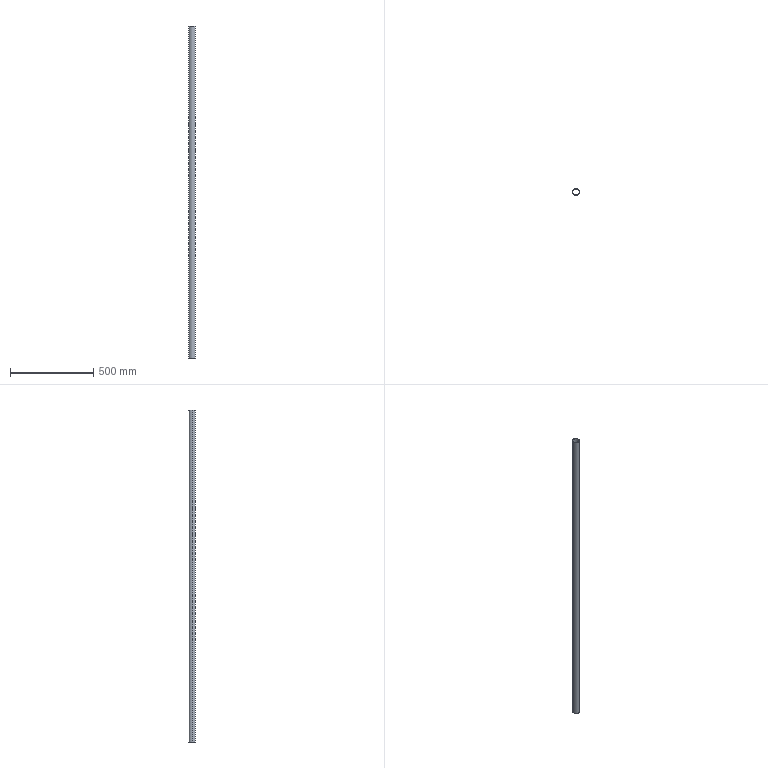Part | SolidWorks | features Extrusion 1 | 1 solid | 6 faces | box 42 x 42 x 2000 mm | volume 502655 mm3 | cylinder 4 | plane 2 | commonest cylinder face diameters 38 x2 42 x2
STEP:
#1=CARTESIAN_POINT('',(-19.,0.,2000.));
#2=VERTEX_POINT('',#1);
#3=CARTESIAN_POINT('',(19.,0.,2000.));
#4=VERTEX_POINT('',#3);
#5=CARTESIAN_POINT('',(0.,0.,2000.));
#6=DIRECTION('',(0.,0.,1.));
#7=DIRECTION('',(1.,0.,0.));
#8=AXIS2_PLACEMENT_3D('',#5,#6,#7);
#9=CIRCLE('',#8,19.);
#10=EDGE_CURVE('',#2,#4,#9,.T.);
#11=ORIENTED_EDGE('',*,*,#10,.T.);
#12=CARTESIAN_POINT('',(19.,0.,0.));
#13=VERTEX_POINT('',#12);
#14=CARTESIAN_POINT('',(19.,0.,2000.));
#15=DIRECTION('',(0.,0.,-1.));
#16=VECTOR('',#15,1000.);
#17=LINE('',#14,#16);
#18=EDGE_CURVE('',#4,#13,#17,.T.);
#19=ORIENTED_EDGE('',*,*,#18,.T.);
#20=CARTESIAN_POINT('',(-19.,0.,0.));
#21=VERTEX_POINT('',#20);
#22=CARTESIAN_POINT('',(0.,0.,0.));
#23=DIRECTION('',(0.,0.,1.));
#24=DIRECTION('',(1.,0.,0.));
#25=AXIS2_PLACEMENT_3D('',#22,#23,#24);
#26=CIRCLE('',#25,19.);
#27=EDGE_CURVE('',#21,#13,#26,.T.);
#28=ORIENTED_EDGE('',*,*,#27,.F.);
#29=CARTESIAN_POINT('',(-19.,0.,2000.));
#30=DIRECTION('',(0.,0.,-1.));
#31=VECTOR('',#30,1000.);
#32=LINE('',#29,#31);
#33=EDGE_CURVE('',#2,#21,#32,.T.);
#34=ORIENTED_EDGE('',*,*,#33,.F.);
#35=EDGE_LOOP('',(#11,#19,#28,#34));
#36=FACE_OUTER_BOUND('',#35,.T.);
#37=CARTESIAN_POINT('',(0.,0.,2000.));
#38=DIRECTION('',(0.,0.,-1.));
#39=DIRECTION('',(-1.,0.,0.));
#40=AXIS2_PLACEMENT_3D('',#37,#38,#39);
#41=CYLINDRICAL_SURFACE('',#40,19.);
#42=ADVANCED_FACE('',(#36),#41,.F.);
#43=CARTESIAN_POINT('',(21.,0.,2000.));
#44=VERTEX_POINT('',#43);
#45=CARTESIAN_POINT('',(-21.,0.,2000.));
#46=VERTEX_POINT('',#45);
#47=CARTESIAN_POINT('',(0.,0.,2000.));
#48=DIRECTION('',(0.,0.,1.));
#49=DIRECTION('',(1.,0.,0.));
#50=AXIS2_PLACEMENT_3D('',#47,#48,#49);
#51=CIRCLE('',#50,21.);
#52=EDGE_CURVE('',#44,#46,#51,.T.);
#53=ORIENTED_EDGE('',*,*,#52,.F.);
#54=CARTESIAN_POINT('',(21.,0.,0.));
#55=VERTEX_POINT('',#54);
#56=CARTESIAN_POINT('',(21.,0.,2000.));
#57=DIRECTION('',(0.,0.,-1.));
#58=VECTOR('',#57,1000.);
#59=LINE('',#56,#58);
#60=EDGE_CURVE('',#44,#55,#59,.T.);
#61=ORIENTED_EDGE('',*,*,#60,.T.);
#62=CARTESIAN_POINT('',(-21.,0.,0.));
#63=VERTEX_POINT('',#62);
#64=CARTESIAN_POINT('',(0.,0.,0.));
#65=DIRECTION('',(0.,0.,1.));
#66=DIRECTION('',(1.,0.,0.));
#67=AXIS2_PLACEMENT_3D('',#64,#65,#66);
#68=CIRCLE('',#67,21.);
#69=EDGE_CURVE('',#55,#63,#68,.T.);
#70=ORIENTED_EDGE('',*,*,#69,.T.);
#71=CARTESIAN_POINT('',(-21.,0.,2000.));
#72=DIRECTION('',(0.,0.,-1.));
#73=VECTOR('',#72,1000.);
#74=LINE('',#71,#73);
#75=EDGE_CURVE('',#46,#63,#74,.T.);
#76=ORIENTED_EDGE('',*,*,#75,.F.);
#77=EDGE_LOOP('',(#53,#61,#70,#76));
#78=FACE_OUTER_BOUND('',#77,.T.);
#79=CARTESIAN_POINT('',(0.,0.,2000.));
#80=DIRECTION('',(0.,0.,-1.));
#81=DIRECTION('',(-1.,0.,0.));
#82=AXIS2_PLACEMENT_3D('',#79,#80,#81);
#83=CYLINDRICAL_SURFACE('',#82,21.);
#84=ADVANCED_FACE('',(#78),#83,.T.);
#85=CARTESIAN_POINT('',(0.,0.,2000.));
#86=DIRECTION('',(0.,0.,1.));
#87=DIRECTION('',(1.,0.,0.));
#88=AXIS2_PLACEMENT_3D('',#85,#86,#87);
#89=CIRCLE('',#88,21.);
#90=EDGE_CURVE('',#46,#44,#89,.T.);
#91=ORIENTED_EDGE('',*,*,#90,.T.);
#92=ORIENTED_EDGE('',*,*,#52,.T.);
#93=EDGE_LOOP('',(#91,#92));
#94=FACE_OUTER_BOUND('',#93,.T.);
#95=ORIENTED_EDGE('',*,*,#10,.F.);
#96=CARTESIAN_POINT('',(0.,0.,2000.));
#97=DIRECTION('',(0.,0.,1.));
#98=DIRECTION('',(1.,0.,0.));
#99=AXIS2_PLACEMENT_3D('',#96,#97,#98);
#100=CIRCLE('',#99,19.);
#101=EDGE_CURVE('',#4,#2,#100,.T.);
#102=ORIENTED_EDGE('',*,*,#101,.F.);
#103=EDGE_LOOP('',(#95,#102));
#104=FACE_BOUND('',#103,.T.);
#105=CARTESIAN_POINT('',(0.,0.,2000.));
#106=DIRECTION('',(0.,0.,1.));
#107=DIRECTION('',(1.,0.,0.));
#108=AXIS2_PLACEMENT_3D('',#105,#106,#107);
#109=PLANE('',#108);
#110=ADVANCED_FACE('',(#94,#104),#109,.T.);
#111=CARTESIAN_POINT('',(0.,0.,0.));
#112=DIRECTION('',(0.,0.,1.));
#113=DIRECTION('',(1.,0.,0.));
#114=AXIS2_PLACEMENT_3D('',#111,#112,#113);
#115=CIRCLE('',#114,21.);
#116=EDGE_CURVE('',#63,#55,#115,.T.);
#117=ORIENTED_EDGE('',*,*,#116,.F.);
#118=ORIENTED_EDGE('',*,*,#69,.F.);
#119=EDGE_LOOP('',(#117,#118));
#120=FACE_OUTER_BOUND('',#119,.T.);
#121=ORIENTED_EDGE('',*,*,#27,.T.);
#122=CARTESIAN_POINT('',(0.,0.,0.));
#123=DIRECTION('',(0.,0.,1.));
#124=DIRECTION('',(1.,0.,0.));
#125=AXIS2_PLACEMENT_3D('',#122,#123,#124);
#126=CIRCLE('',#125,19.);
#127=EDGE_CURVE('',#13,#21,#126,.T.);
#128=ORIENTED_EDGE('',*,*,#127,.T.);
#129=EDGE_LOOP('',(#121,#128));
#130=FACE_BOUND('',#129,.T.);
#131=CARTESIAN_POINT('',(0.,0.,0.));
#132=DIRECTION('',(0.,0.,1.));
#133=DIRECTION('',(1.,0.,0.));
#134=AXIS2_PLACEMENT_3D('',#131,#132,#133);
#135=PLANE('',#134);
#136=ADVANCED_FACE('',(#120,#130),#135,.F.);
#137=ORIENTED_EDGE('',*,*,#60,.F.);
#138=ORIENTED_EDGE('',*,*,#90,.F.);
#139=ORIENTED_EDGE('',*,*,#75,.T.);
#140=ORIENTED_EDGE('',*,*,#116,.T.);
#141=EDGE_LOOP('',(#137,#138,#139,#140));
#142=FACE_OUTER_BOUND('',#141,.T.);
#143=CARTESIAN_POINT('',(0.,0.,2000.));
#144=DIRECTION('',(0.,0.,-1.));
#145=DIRECTION('',(-1.,0.,0.));
#146=AXIS2_PLACEMENT_3D('',#143,#144,#145);
#147=CYLINDRICAL_SURFACE('',#146,21.);
#148=ADVANCED_FACE('',(#142),#147,.T.);
#149=ORIENTED_EDGE('',*,*,#18,.F.);
#150=ORIENTED_EDGE('',*,*,#101,.T.);
#151=ORIENTED_EDGE('',*,*,#33,.T.);
#152=ORIENTED_EDGE('',*,*,#127,.F.);
#153=EDGE_LOOP('',(#149,#150,#151,#152));
#154=FACE_OUTER_BOUND('',#153,.T.);
#155=CARTESIAN_POINT('',(0.,0.,2000.));
#156=DIRECTION('',(0.,0.,-1.));
#157=DIRECTION('',(-1.,0.,0.));
#158=AXIS2_PLACEMENT_3D('',#155,#156,#157);
#159=CYLINDRICAL_SURFACE('',#158,19.);
#160=ADVANCED_FACE('',(#154),#159,.F.);
#161=CLOSED_SHELL('',(#42,#84,#110,#136,#148,#160));
#162=MANIFOLD_SOLID_BREP('',#161);
#163=CARTESIAN_POINT('',(0.,0.,0.));
#164=DIRECTION('',(0.,0.,1.));
#165=DIRECTION('',(1.,0.,0.));
#166=AXIS2_PLACEMENT_3D('',#163,#164,#165);
#167=(LENGTH_UNIT()NAMED_UNIT(*)SI_UNIT(.MILLI.,.METRE.));
#168=UNCERTAINTY_MEASURE_WITH_UNIT(LENGTH_MEASURE(0.00001),#167,'','');
#169=(NAMED_UNIT(*)PLANE_ANGLE_UNIT()SI_UNIT($,.RADIAN.));
#170=(NAMED_UNIT(*)SI_UNIT($,.STERADIAN.)SOLID_ANGLE_UNIT());
#171=(GEOMETRIC_REPRESENTATION_CONTEXT(3)GLOBAL_UNCERTAINTY_ASSIGNED_CONTEXT((#168))GLOBAL_UNIT_ASSIGNED_CONTEXT((#167,#169,#170))REPRESENTATION_CONTEXT('',''));
#172=ADVANCED_BREP_SHAPE_REPRESENTATION('',(#162,#166),#171);